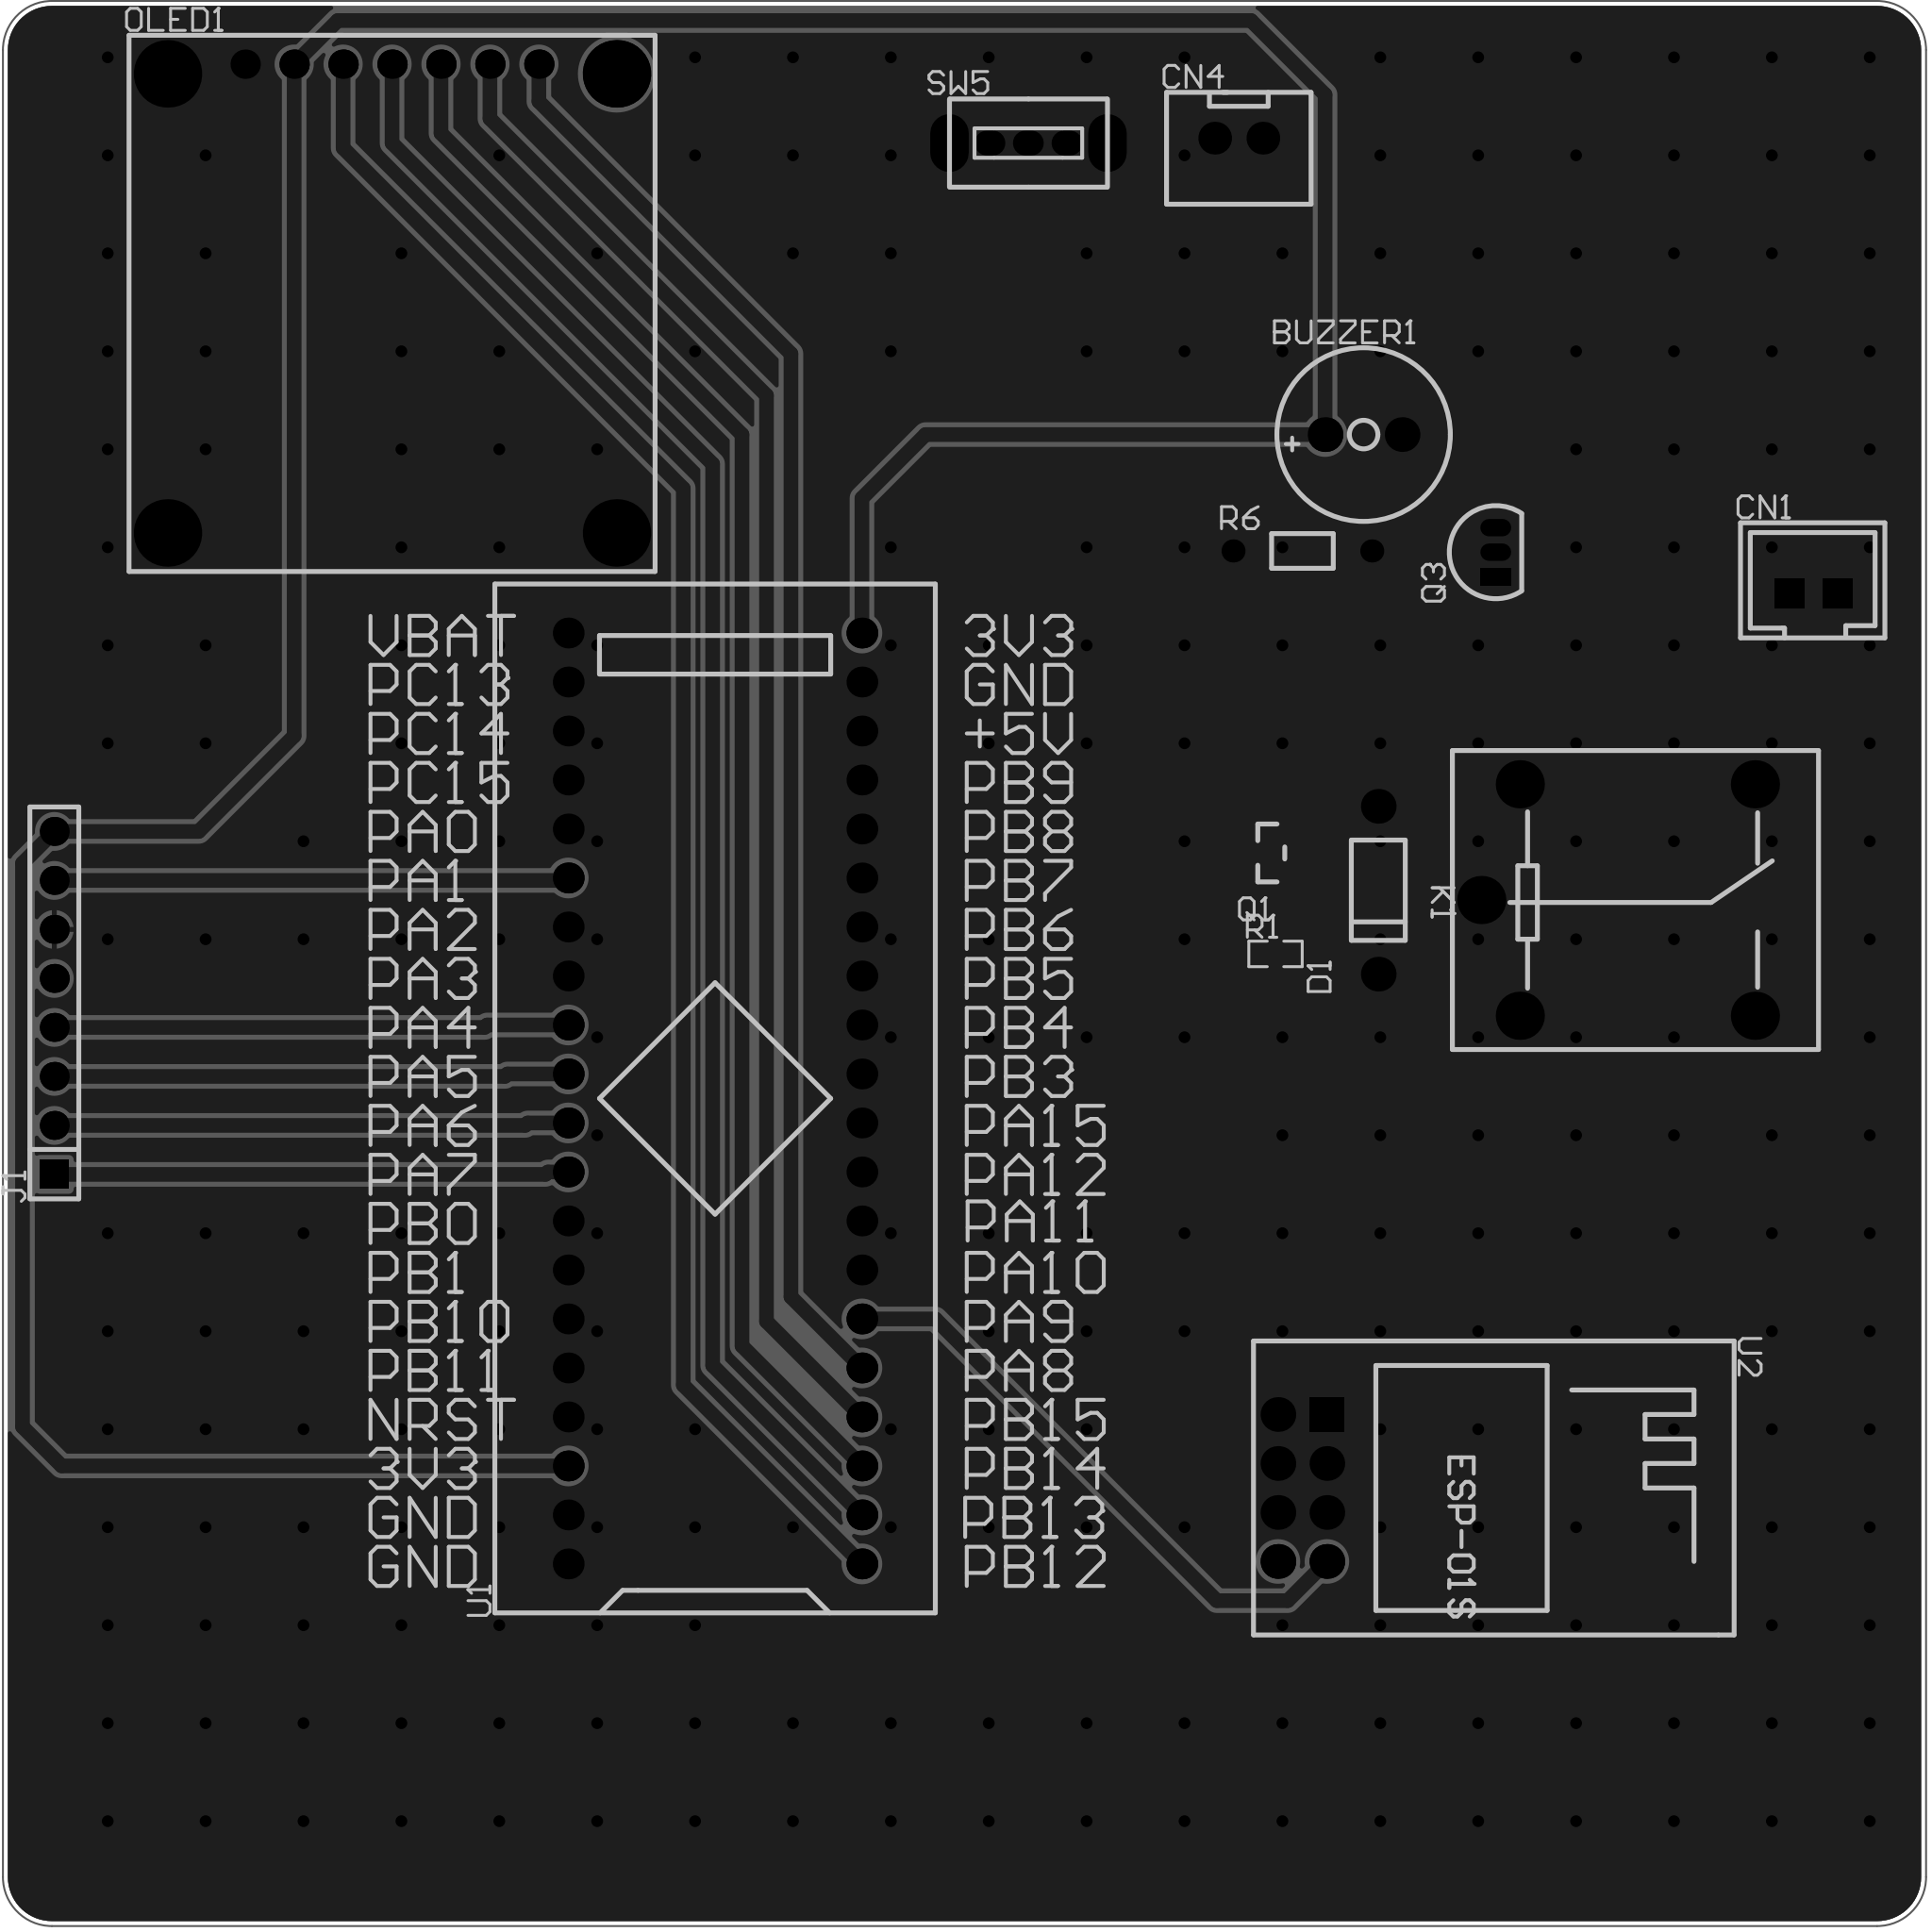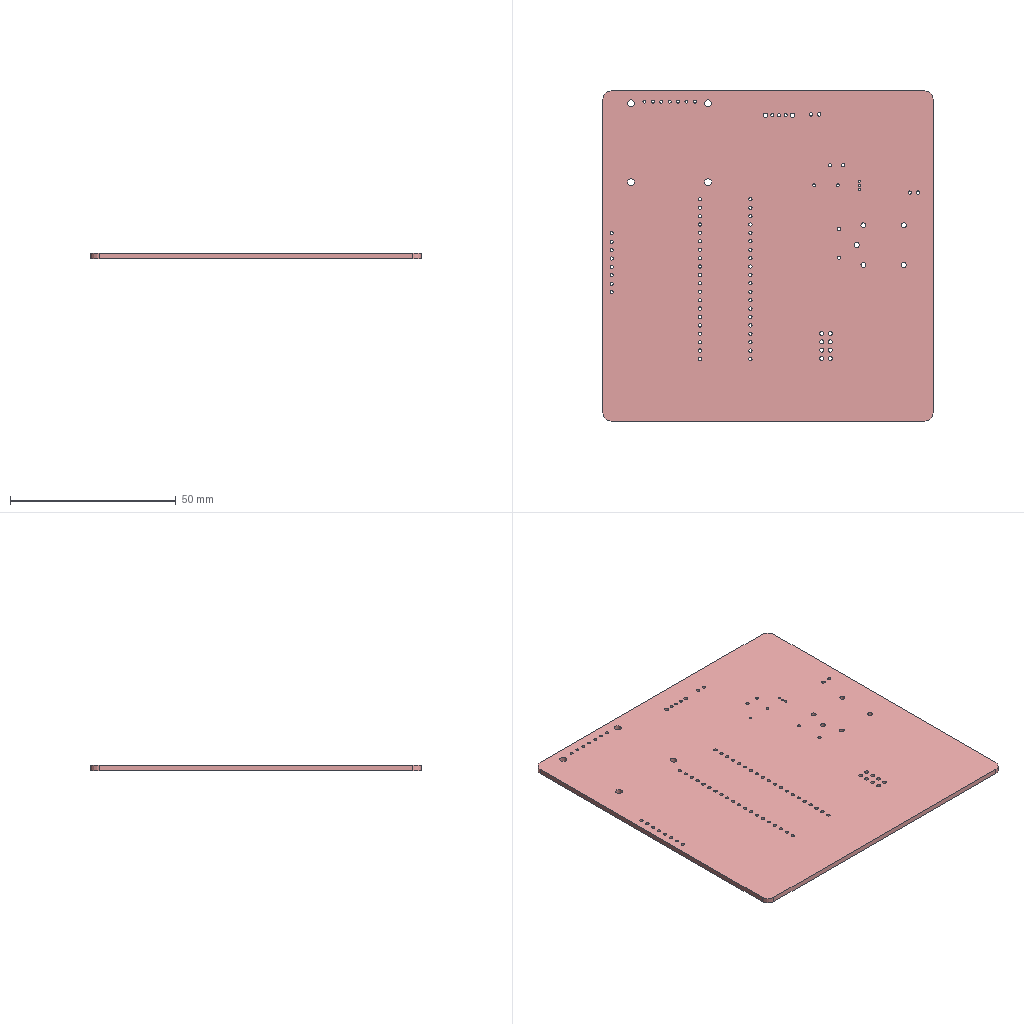Circuit board layout | Altium Designer | box 99.8 x 99.8 x 1.6 mm
Layer stack:
# Altium Designer layer stack of  (unit mm; dielectric type: 0 none, 1 core, 2 prepreg, 3 surface material)
index,name,kind,layer,copper_thickness_mm,dielectric_type,dielectric_thickness_mm,dielectric_material,dielectric_constant
0,Top Paste Mask Layer,other,,,,,,
1,Top Silkscreen Layer,other,,,,,,
2,Top Solder Mask Layer,dielectric,,,3,0.01,,3.3
3,Top Layer,copper,Top Layer,0.035,,,,
4,Dielectric1,dielectric,,,3,1.51,FR4,4.5
5,Bottom Layer,copper,Bottom Layer,0.035,,,,
6,Bottom Solder Mask Layer,dielectric,,,3,0.01,,3.3
7,Bottom Silkscreen Layer,other,,,,,,
8,Bottom Paste Mask Layer,other,,,,,,
# drill layer pairs: low layer,high layer
drill_pair,Top Layer,Bottom Layer
Part placement:
Designator,Comment,Layer,Footprint,Center-X(mm),Center-Y(mm),Rotation
BUZZER1,2.7kHz,TopLayer,BUZ-TH_BD9.0-P4.00-D0.6-FD,155.194,169.418,0
J1,,TopLayer,HDR-TH_8P-P2.54-V-M,87.249,139.954,90
U1,LCKFB-DKX-STM32F103C8T6,TopLayer,CONN-TH_L53.3-W22.9_STM32F103C8T6-CARD,121.539,135.001,90
OLED1,,TopLayer,0.96OLED,104.775,176.469,0
R6,1K,TopLayer,Res_1/8W,152.019,163.385,0
Q3,,TopLayer,S8050_TO_92,162.052,163.322,90
U2,ESP-01S,TopLayer,WIFIM-TH_ESP-01S,152.019,114.808,270
CN1,XH2.54-2PIN-straight pin,TopLayer,CONN-TH_XH2.54-2P,178.562,161.163,0
D1,,TopLayer,DO_1N4007,155.956,145.796,90
K1,HT3F-5VDC-SHG,TopLayer,RELAY-TH_HT3F-DCXX-X-X,168.402,145.288,0
Q1,,TopLayer,S8050_SOT-23,150.402,147.728,0
R1,1K,TopLayer,R0603,150.622,142.494,0
CN4,XH2.54*2P_through-hole,TopLayer,CONN-TH_2P-P2.50-XH2.54-2P,148.717,184.785,0
SW5,,TopLayer,拨动开关,137.803,184.531,0
Pad and via stacks:
# Altium Designer via and pad stacks of  (unit mm). Each distinct definition once, with the count of objects using it.
# via: kind,start_layer,end_layer,hole_mm,diameter_mm,mode(0 simple;1 top-mid-bottom;2 full stack),diameter_per_layer,count,example_net
# pad: kind,layer,hole_mm,hole_type(0 round;1 square;2 slot),plating,top_size,top_shape(1 round;2 rect;3 octagon;9 rounded rect),mid_size,bottom_size,mode,footprint,size_per_layer,count,example
pad,Multi-Layer,1,0,plated,1.8x1.8,1,1.8x1.8,1.8x1.8,0,BUZ-TH_BD9.0-P4.00-D0.6-FD,,2,BUZZER1.1
pad,Multi-Layer,1,0,plated,1.5x1.5,2,1.5x1.5,1.5x1.5,0,HDR-TH_8P-P2.54-V-M,,1,J1.1
pad,Multi-Layer,1,0,plated,1.5x1.5,1,1.5x1.5,1.5x1.5,0,HDR-TH_8P-P2.54-V-M,,7,J1.2
pad,Multi-Layer,1,0,plated,1.6x1.6,1,1.6x1.6,1.6x1.6,0,CONN-TH_L53.3-W22.9_STM32F103C8T6-CARD,,40,U1.1
pad,Multi-Layer,0.9144,0,plated,1.524x1.524,1,1.524x1.524,1.524x1.524,0,0.96OLED,,7,OLED1.1
pad,Multi-Layer,2.1,0,plated,3.5x3.5,1,3.5x3.5,3.5x3.5,0,0.96OLED,,4,OLED1.0
pad,Multi-Layer,0.8001,0,plated,1.199x1.199,1,1.199x1.199,1.199x1.199,0,Res_1/8W,,2,R6.1
pad,Multi-Layer,0.701,0,plated,0.8992x1.6,2,0.8992x1.6,0.8992x1.6,0,S8050_TO_92,,1,Q3.1
pad,Multi-Layer,0.701,0,plated,0.8992x1.6,1,0.8992x1.6,0.8992x1.6,0,S8050_TO_92,,2,Q3.2
pad,Multi-Layer,1.2,0,plated,1.8x1.8,2,1.8x1.8,1.8x1.8,0,WIFIM-TH_ESP-01S,,1,U2.1
pad,Multi-Layer,1.2,0,plated,1.8x1.8,1,1.8x1.8,1.8x1.8,0,WIFIM-TH_ESP-01S,,7,U2.2
pad,Multi-Layer,1,2,plated,1.524x1.524,2,1.524x1.524,1.524x1.524,0,CONN-TH_XH2.54-2P,,2,CN1.1
pad,Multi-Layer,1,0,plated,1.8x1.8,1,1.8x1.8,1.8x1.8,0,DO_1N4007,,2,D1.1
pad,Multi-Layer,1.5,0,plated,2.5x2.5,1,2.5x2.5,2.5x2.5,0,RELAY-TH_HT3F-DCXX-X-X,,5,K1.1
pad,Multi-Layer,1.05,0,plated,1.7x1.7,1,1.7x1.7,1.7x1.7,0,CONN-TH_2P-P2.50-XH2.54-2P,,2,CN4.2
pad,Multi-Layer,0.8992,0,plated,1.6x1.3,1,1.6x1.3,1.6x1.3,0,\u00B2\u00A6\u00B6\u00AF\u00BF\u00AA\u00B9\u00D8,,3,SW5.1
pad,Multi-Layer,1.3,0,plated,3x1.999,1,3x1.999,3x1.999,0,\u00B2\u00A6\u00B6\u00AF\u00BF\u00AA\u00B9\u00D8,,2,SW5.4
pad,Top Layer,0,0,plated,1x0.8,2,1x0.8,1x0.8,0,S8050_SOT-23,,3,Q1.2
pad,Top Layer,0,0,plated,0.8065x0.864,2,0.8065x0.864,0.8065x0.864,0,R0603,,2,R1.2
via,Top Layer,Bottom Layer,0.3048,0.61,0,,271,GND
Copper pours:
name,layer,net,type(0 solid;1 hatched;2 none)
Top Layer-GND,Top Layer,GND,0
Bottom Layer-GND,Bottom Layer,GND,0
Bottom Layer-GND 1,Bottom Layer,GND,0